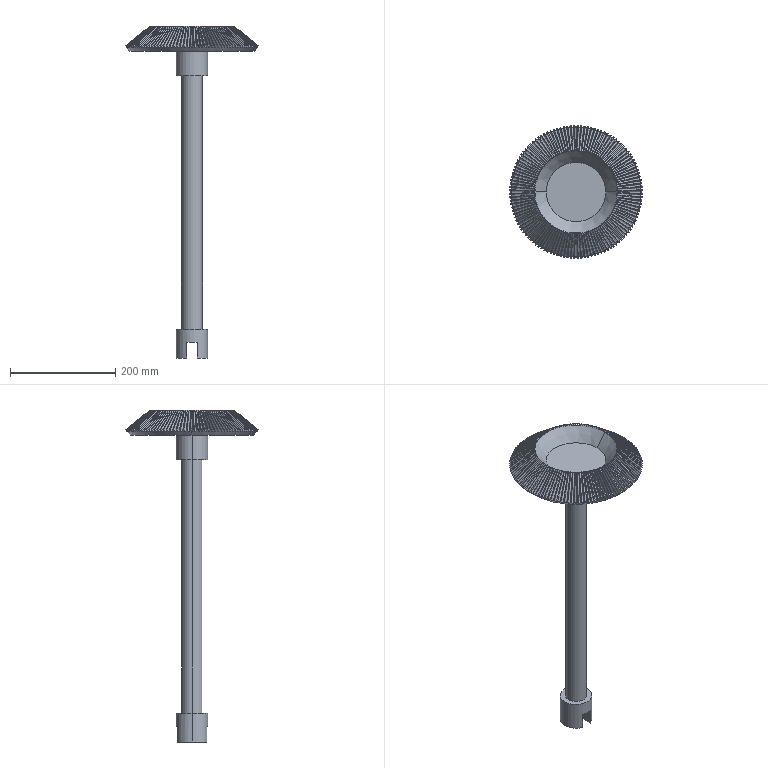Part | SolidWorks | 1 solid | 259 faces | box 252.245 x 252.245 x 629.793 mm | volume 2125669 mm3 | cone 124 | spline 120 | plane 9 | cylinder 6 | commonest cylinder face diameters 60 x4 40 x2